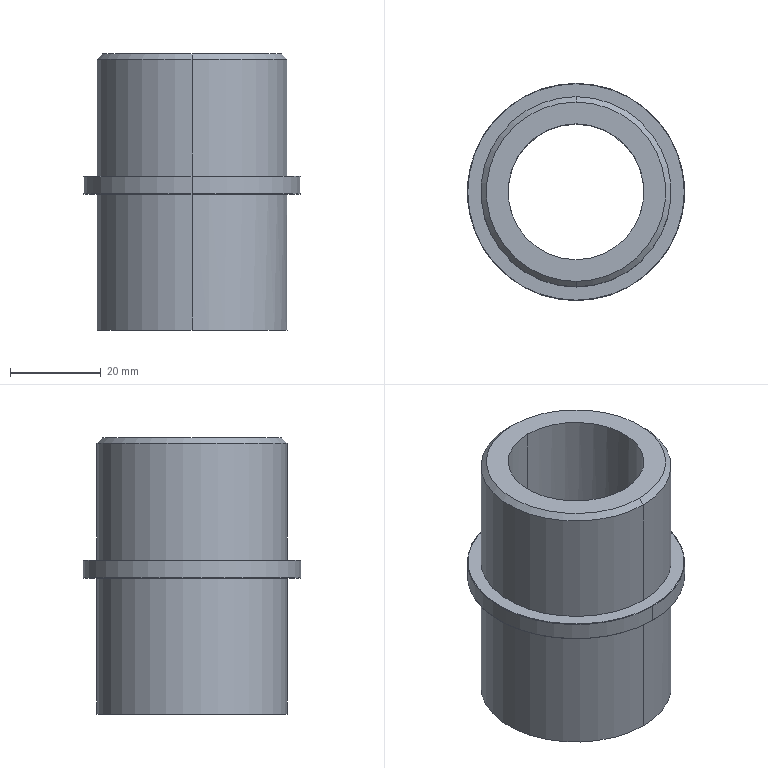Part | Creo | 1 solid | 18 faces | box 48 x 48 x 61 mm | volume 42995 mm3 | cylinder 8 | cone 6 | plane 4 | commonest cylinder face diameters 42 x4 30 x2 48 x2
STEP:
#1=CARTESIAN_POINT('',(166.,209.995,-326.));
#2=VERTEX_POINT('',#1);
#3=CARTESIAN_POINT('',(145.,188.995,-326.));
#4=VERTEX_POINT('',#3);
#5=CARTESIAN_POINT('',(145.,209.995,-326.));
#6=DIRECTION('',(0.,0.,-1.));
#7=DIRECTION('',(1.,0.,0.));
#8=AXIS2_PLACEMENT_3D('',#5,#6,#7);
#9=CIRCLE('',#8,21.);
#10=EDGE_CURVE('',#2,#4,#9,.T.);
#11=ORIENTED_EDGE('',*,*,#10,.F.);
#12=CARTESIAN_POINT('',(145.,230.995,-326.));
#13=VERTEX_POINT('',#12);
#14=CARTESIAN_POINT('',(145.,209.995,-326.));
#15=DIRECTION('',(0.,0.,-1.));
#16=DIRECTION('',(0.,1.,0.));
#17=AXIS2_PLACEMENT_3D('',#14,#15,#16);
#18=CIRCLE('',#17,21.);
#19=EDGE_CURVE('',#13,#2,#18,.T.);
#20=ORIENTED_EDGE('',*,*,#19,.F.);
#21=CARTESIAN_POINT('',(145.,209.995,-326.));
#22=DIRECTION('',(0.,0.,-1.));
#23=DIRECTION('',(0.,-1.,0.));
#24=AXIS2_PLACEMENT_3D('',#21,#22,#23);
#25=CIRCLE('',#24,21.);
#26=EDGE_CURVE('',#4,#13,#25,.T.);
#27=ORIENTED_EDGE('',*,*,#26,.F.);
#28=EDGE_LOOP('',(#11,#20,#27));
#29=FACE_OUTER_BOUND('',#28,.F.);
#30=CARTESIAN_POINT('',(160.,209.995,-326.));
#31=VERTEX_POINT('',#30);
#32=CARTESIAN_POINT('',(145.,224.995,-326.));
#33=VERTEX_POINT('',#32);
#34=CARTESIAN_POINT('',(145.,209.995,-326.));
#35=DIRECTION('',(0.,0.,1.));
#36=DIRECTION('',(1.,0.,0.));
#37=AXIS2_PLACEMENT_3D('',#34,#35,#36);
#38=CIRCLE('',#37,15.);
#39=EDGE_CURVE('',#31,#33,#38,.T.);
#40=ORIENTED_EDGE('',*,*,#39,.F.);
#41=CARTESIAN_POINT('',(145.,194.995,-326.));
#42=VERTEX_POINT('',#41);
#43=CARTESIAN_POINT('',(145.,209.995,-326.));
#44=DIRECTION('',(0.,0.,1.));
#45=DIRECTION('',(0.,-1.,0.));
#46=AXIS2_PLACEMENT_3D('',#43,#44,#45);
#47=CIRCLE('',#46,15.);
#48=EDGE_CURVE('',#42,#31,#47,.T.);
#49=ORIENTED_EDGE('',*,*,#48,.F.);
#50=CARTESIAN_POINT('',(130.,209.995,-326.));
#51=VERTEX_POINT('',#50);
#52=CARTESIAN_POINT('',(145.,209.995,-326.));
#53=DIRECTION('',(0.,0.,1.));
#54=DIRECTION('',(-1.,0.,0.));
#55=AXIS2_PLACEMENT_3D('',#52,#53,#54);
#56=CIRCLE('',#55,15.);
#57=EDGE_CURVE('',#51,#42,#56,.T.);
#58=ORIENTED_EDGE('',*,*,#57,.F.);
#59=CARTESIAN_POINT('',(145.,209.995,-326.));
#60=DIRECTION('',(0.,0.,1.));
#61=DIRECTION('',(0.,1.,0.));
#62=AXIS2_PLACEMENT_3D('',#59,#60,#61);
#63=CIRCLE('',#62,15.);
#64=EDGE_CURVE('',#33,#51,#63,.T.);
#65=ORIENTED_EDGE('',*,*,#64,.F.);
#66=EDGE_LOOP('',(#40,#49,#58,#65));
#67=FACE_BOUND('',#66,.F.);
#68=CARTESIAN_POINT('',(45.,-0.004699,-326.));
#69=DIRECTION('',(0.,0.,1.));
#70=DIRECTION('',(0.,1.,0.));
#71=AXIS2_PLACEMENT_3D('',#68,#69,#70);
#72=PLANE('',#71);
#73=ADVANCED_FACE('',(#29,#67),#72,.F.);
#74=CARTESIAN_POINT('',(145.,188.995,-296.));
#75=VERTEX_POINT('',#74);
#76=CARTESIAN_POINT('',(145.,230.995,-296.));
#77=VERTEX_POINT('',#76);
#78=CARTESIAN_POINT('',(145.,209.995,-296.));
#79=DIRECTION('',(0.,0.,1.));
#80=DIRECTION('',(0.,-1.,0.));
#81=AXIS2_PLACEMENT_3D('',#78,#79,#80);
#82=CIRCLE('',#81,21.);
#83=EDGE_CURVE('',#75,#77,#82,.T.);
#84=ORIENTED_EDGE('',*,*,#83,.T.);
#85=CARTESIAN_POINT('',(145.,230.995,-296.));
#86=DIRECTION('',(0.,0.,-1.));
#87=VECTOR('',#86,30.);
#88=LINE('',#85,#87);
#89=EDGE_CURVE('',#77,#13,#88,.T.);
#90=ORIENTED_EDGE('',*,*,#89,.T.);
#91=ORIENTED_EDGE('',*,*,#19,.T.);
#92=ORIENTED_EDGE('',*,*,#10,.T.);
#93=CARTESIAN_POINT('',(145.,188.995,-296.));
#94=DIRECTION('',(0.,0.,-1.));
#95=VECTOR('',#94,30.);
#96=LINE('',#93,#95);
#97=EDGE_CURVE('',#75,#4,#96,.T.);
#98=ORIENTED_EDGE('',*,*,#97,.F.);
#99=EDGE_LOOP('',(#84,#90,#91,#92,#98));
#100=FACE_OUTER_BOUND('',#99,.F.);
#101=CARTESIAN_POINT('',(145.,209.995,-262.35));
#102=DIRECTION('',(0.,0.,-1.));
#103=DIRECTION('',(0.,-1.,0.));
#104=AXIS2_PLACEMENT_3D('',#101,#102,#103);
#105=CYLINDRICAL_SURFACE('',#104,21.);
#106=ADVANCED_FACE('',(#100),#105,.T.);
#107=CARTESIAN_POINT('',(145.,186.095,-296.));
#108=VERTEX_POINT('',#107);
#109=CARTESIAN_POINT('',(145.,233.895,-296.));
#110=VERTEX_POINT('',#109);
#111=CARTESIAN_POINT('',(145.,209.995,-296.));
#112=DIRECTION('',(0.,0.,-1.));
#113=DIRECTION('',(0.,-1.,0.));
#114=AXIS2_PLACEMENT_3D('',#111,#112,#113);
#115=CIRCLE('',#114,23.9);
#116=EDGE_CURVE('',#108,#110,#115,.T.);
#117=ORIENTED_EDGE('',*,*,#116,.F.);
#118=CARTESIAN_POINT('',(145.,209.995,-296.));
#119=DIRECTION('',(0.,0.,-1.));
#120=DIRECTION('',(0.,1.,0.));
#121=AXIS2_PLACEMENT_3D('',#118,#119,#120);
#122=CIRCLE('',#121,23.9);
#123=EDGE_CURVE('',#110,#108,#122,.T.);
#124=ORIENTED_EDGE('',*,*,#123,.F.);
#125=EDGE_LOOP('',(#117,#124));
#126=FACE_OUTER_BOUND('',#125,.F.);
#127=ORIENTED_EDGE('',*,*,#83,.F.);
#128=CARTESIAN_POINT('',(145.,209.995,-296.));
#129=DIRECTION('',(0.,0.,1.));
#130=DIRECTION('',(0.,1.,0.));
#131=AXIS2_PLACEMENT_3D('',#128,#129,#130);
#132=CIRCLE('',#131,21.);
#133=EDGE_CURVE('',#77,#75,#132,.T.);
#134=ORIENTED_EDGE('',*,*,#133,.F.);
#135=EDGE_LOOP('',(#127,#134));
#136=FACE_BOUND('',#135,.F.);
#137=CARTESIAN_POINT('',(145.,209.995,-296.));
#138=DIRECTION('',(0.,0.,-1.));
#139=DIRECTION('',(0.,-1.,0.));
#140=AXIS2_PLACEMENT_3D('',#137,#138,#139);
#141=PLANE('',#140);
#142=ADVANCED_FACE('',(#126,#136),#141,.T.);
#143=ORIENTED_EDGE('',*,*,#133,.T.);
#144=ORIENTED_EDGE('',*,*,#97,.T.);
#145=ORIENTED_EDGE('',*,*,#26,.T.);
#146=ORIENTED_EDGE('',*,*,#89,.F.);
#147=EDGE_LOOP('',(#143,#144,#145,#146));
#148=FACE_OUTER_BOUND('',#147,.F.);
#149=CARTESIAN_POINT('',(145.,209.995,-262.35));
#150=DIRECTION('',(0.,0.,-1.));
#151=DIRECTION('',(0.,-1.,0.));
#152=AXIS2_PLACEMENT_3D('',#149,#150,#151);
#153=CYLINDRICAL_SURFACE('',#152,21.);
#154=ADVANCED_FACE('',(#148),#153,.T.);
#155=CARTESIAN_POINT('',(145.,185.995,-295.9));
#156=VERTEX_POINT('',#155);
#157=CARTESIAN_POINT('',(145.,233.995,-295.9));
#158=VERTEX_POINT('',#157);
#159=CARTESIAN_POINT('',(145.,209.995,-295.9));
#160=DIRECTION('',(0.,0.,-1.));
#161=DIRECTION('',(0.,-1.,0.));
#162=AXIS2_PLACEMENT_3D('',#159,#160,#161);
#163=CIRCLE('',#162,24.);
#164=EDGE_CURVE('',#156,#158,#163,.T.);
#165=ORIENTED_EDGE('',*,*,#164,.F.);
#166=CARTESIAN_POINT('',(145.,186.095,-296.));
#167=DIRECTION('',(0.,-0.7071,0.7071));
#168=VECTOR('',#167,0.1414);
#169=LINE('',#166,#168);
#170=EDGE_CURVE('',#108,#156,#169,.T.);
#171=ORIENTED_EDGE('',*,*,#170,.F.);
#172=ORIENTED_EDGE('',*,*,#116,.T.);
#173=CARTESIAN_POINT('',(145.,233.895,-296.));
#174=DIRECTION('',(0.,0.7071,0.7071));
#175=VECTOR('',#174,0.1414);
#176=LINE('',#173,#175);
#177=EDGE_CURVE('',#110,#158,#176,.T.);
#178=ORIENTED_EDGE('',*,*,#177,.T.);
#179=EDGE_LOOP('',(#165,#171,#172,#178));
#180=FACE_OUTER_BOUND('',#179,.F.);
#181=CARTESIAN_POINT('',(145.,209.995,-295.95));
#182=DIRECTION('',(0.,0.,1.));
#183=DIRECTION('',(0.,1.,0.));
#184=AXIS2_PLACEMENT_3D('',#181,#182,#183);
#185=CONICAL_SURFACE('',#184,23.95,45.);
#186=ADVANCED_FACE('',(#180),#185,.T.);
#187=CARTESIAN_POINT('',(145.,233.995,-292.1));
#188=VERTEX_POINT('',#187);
#189=CARTESIAN_POINT('',(145.,185.995,-292.1));
#190=VERTEX_POINT('',#189);
#191=CARTESIAN_POINT('',(145.,209.995,-292.1));
#192=DIRECTION('',(0.,0.,1.));
#193=DIRECTION('',(0.,1.,0.));
#194=AXIS2_PLACEMENT_3D('',#191,#192,#193);
#195=CIRCLE('',#194,24.);
#196=EDGE_CURVE('',#188,#190,#195,.T.);
#197=ORIENTED_EDGE('',*,*,#196,.T.);
#198=CARTESIAN_POINT('',(145.,185.995,-292.1));
#199=DIRECTION('',(0.,0.,-1.));
#200=VECTOR('',#199,3.8);
#201=LINE('',#198,#200);
#202=EDGE_CURVE('',#190,#156,#201,.T.);
#203=ORIENTED_EDGE('',*,*,#202,.T.);
#204=ORIENTED_EDGE('',*,*,#164,.T.);
#205=CARTESIAN_POINT('',(145.,233.995,-292.1));
#206=DIRECTION('',(0.,0.,-1.));
#207=VECTOR('',#206,3.8);
#208=LINE('',#205,#207);
#209=EDGE_CURVE('',#188,#158,#208,.T.);
#210=ORIENTED_EDGE('',*,*,#209,.F.);
#211=EDGE_LOOP('',(#197,#203,#204,#210));
#212=FACE_OUTER_BOUND('',#211,.F.);
#213=CARTESIAN_POINT('',(145.,209.995,-262.35));
#214=DIRECTION('',(0.,0.,-1.));
#215=DIRECTION('',(0.,-1.,0.));
#216=AXIS2_PLACEMENT_3D('',#213,#214,#215);
#217=CYLINDRICAL_SURFACE('',#216,24.);
#218=ADVANCED_FACE('',(#212),#217,.T.);
#219=ORIENTED_EDGE('',*,*,#196,.F.);
#220=CARTESIAN_POINT('',(145.,233.895,-292.));
#221=VERTEX_POINT('',#220);
#222=CARTESIAN_POINT('',(145.,233.895,-292.));
#223=DIRECTION('',(0.,0.7071,-0.7071));
#224=VECTOR('',#223,0.1414);
#225=LINE('',#222,#224);
#226=EDGE_CURVE('',#221,#188,#225,.T.);
#227=ORIENTED_EDGE('',*,*,#226,.F.);
#228=CARTESIAN_POINT('',(145.,186.095,-292.));
#229=VERTEX_POINT('',#228);
#230=CARTESIAN_POINT('',(145.,209.995,-292.));
#231=DIRECTION('',(0.,0.,1.));
#232=DIRECTION('',(0.,1.,0.));
#233=AXIS2_PLACEMENT_3D('',#230,#231,#232);
#234=CIRCLE('',#233,23.9);
#235=EDGE_CURVE('',#221,#229,#234,.T.);
#236=ORIENTED_EDGE('',*,*,#235,.T.);
#237=CARTESIAN_POINT('',(145.,186.095,-292.));
#238=DIRECTION('',(0.,-0.7071,-0.7071));
#239=VECTOR('',#238,0.1414);
#240=LINE('',#237,#239);
#241=EDGE_CURVE('',#229,#190,#240,.T.);
#242=ORIENTED_EDGE('',*,*,#241,.T.);
#243=EDGE_LOOP('',(#219,#227,#236,#242));
#244=FACE_OUTER_BOUND('',#243,.F.);
#245=CARTESIAN_POINT('',(145.,209.995,-292.05));
#246=DIRECTION('',(0.,0.,-1.));
#247=DIRECTION('',(0.,-1.,0.));
#248=AXIS2_PLACEMENT_3D('',#245,#246,#247);
#249=CONICAL_SURFACE('',#248,23.95,45.);
#250=ADVANCED_FACE('',(#244),#249,.T.);
#251=CARTESIAN_POINT('',(145.,209.995,-292.1));
#252=DIRECTION('',(0.,0.,1.));
#253=DIRECTION('',(0.,-1.,0.));
#254=AXIS2_PLACEMENT_3D('',#251,#252,#253);
#255=CIRCLE('',#254,24.);
#256=EDGE_CURVE('',#190,#188,#255,.T.);
#257=ORIENTED_EDGE('',*,*,#256,.F.);
#258=ORIENTED_EDGE('',*,*,#241,.F.);
#259=CARTESIAN_POINT('',(145.,209.995,-292.));
#260=DIRECTION('',(0.,0.,1.));
#261=DIRECTION('',(0.,-1.,0.));
#262=AXIS2_PLACEMENT_3D('',#259,#260,#261);
#263=CIRCLE('',#262,23.9);
#264=EDGE_CURVE('',#229,#221,#263,.T.);
#265=ORIENTED_EDGE('',*,*,#264,.T.);
#266=ORIENTED_EDGE('',*,*,#226,.T.);
#267=EDGE_LOOP('',(#257,#258,#265,#266));
#268=FACE_OUTER_BOUND('',#267,.F.);
#269=CARTESIAN_POINT('',(145.,209.995,-292.05));
#270=DIRECTION('',(0.,0.,-1.));
#271=DIRECTION('',(0.,-1.,0.));
#272=AXIS2_PLACEMENT_3D('',#269,#270,#271);
#273=CONICAL_SURFACE('',#272,23.95,45.);
#274=ADVANCED_FACE('',(#268),#273,.T.);
#275=ORIENTED_EDGE('',*,*,#256,.T.);
#276=ORIENTED_EDGE('',*,*,#209,.T.);
#277=CARTESIAN_POINT('',(145.,209.995,-295.9));
#278=DIRECTION('',(0.,0.,-1.));
#279=DIRECTION('',(0.,1.,0.));
#280=AXIS2_PLACEMENT_3D('',#277,#278,#279);
#281=CIRCLE('',#280,24.);
#282=EDGE_CURVE('',#158,#156,#281,.T.);
#283=ORIENTED_EDGE('',*,*,#282,.T.);
#284=ORIENTED_EDGE('',*,*,#202,.F.);
#285=EDGE_LOOP('',(#275,#276,#283,#284));
#286=FACE_OUTER_BOUND('',#285,.F.);
#287=CARTESIAN_POINT('',(145.,209.995,-262.35));
#288=DIRECTION('',(0.,0.,-1.));
#289=DIRECTION('',(0.,-1.,0.));
#290=AXIS2_PLACEMENT_3D('',#287,#288,#289);
#291=CYLINDRICAL_SURFACE('',#290,24.);
#292=ADVANCED_FACE('',(#286),#291,.T.);
#293=ORIENTED_EDGE('',*,*,#282,.F.);
#294=ORIENTED_EDGE('',*,*,#177,.F.);
#295=ORIENTED_EDGE('',*,*,#123,.T.);
#296=ORIENTED_EDGE('',*,*,#170,.T.);
#297=EDGE_LOOP('',(#293,#294,#295,#296));
#298=FACE_OUTER_BOUND('',#297,.F.);
#299=CARTESIAN_POINT('',(145.,209.995,-295.95));
#300=DIRECTION('',(0.,0.,1.));
#301=DIRECTION('',(0.,1.,0.));
#302=AXIS2_PLACEMENT_3D('',#299,#300,#301);
#303=CONICAL_SURFACE('',#302,23.95,45.);
#304=ADVANCED_FACE('',(#298),#303,.T.);
#305=ORIENTED_EDGE('',*,*,#264,.F.);
#306=ORIENTED_EDGE('',*,*,#235,.F.);
#307=EDGE_LOOP('',(#305,#306));
#308=FACE_OUTER_BOUND('',#307,.F.);
#309=CARTESIAN_POINT('',(145.,188.995,-292.));
#310=VERTEX_POINT('',#309);
#311=CARTESIAN_POINT('',(145.,230.995,-292.));
#312=VERTEX_POINT('',#311);
#313=CARTESIAN_POINT('',(145.,209.995,-292.));
#314=DIRECTION('',(0.,0.,-1.));
#315=DIRECTION('',(0.,-1.,0.));
#316=AXIS2_PLACEMENT_3D('',#313,#314,#315);
#317=CIRCLE('',#316,21.);
#318=EDGE_CURVE('',#310,#312,#317,.T.);
#319=ORIENTED_EDGE('',*,*,#318,.F.);
#320=CARTESIAN_POINT('',(145.,209.995,-292.));
#321=DIRECTION('',(0.,0.,-1.));
#322=DIRECTION('',(0.,1.,0.));
#323=AXIS2_PLACEMENT_3D('',#320,#321,#322);
#324=CIRCLE('',#323,21.);
#325=EDGE_CURVE('',#312,#310,#324,.T.);
#326=ORIENTED_EDGE('',*,*,#325,.F.);
#327=EDGE_LOOP('',(#319,#326));
#328=FACE_BOUND('',#327,.F.);
#329=CARTESIAN_POINT('',(145.,209.995,-292.));
#330=DIRECTION('',(0.,0.,-1.));
#331=DIRECTION('',(0.,-1.,0.));
#332=AXIS2_PLACEMENT_3D('',#329,#330,#331);
#333=PLANE('',#332);
#334=ADVANCED_FACE('',(#308,#328),#333,.F.);
#335=CARTESIAN_POINT('',(145.,230.995,-266.2));
#336=VERTEX_POINT('',#335);
#337=CARTESIAN_POINT('',(145.,188.995,-266.2));
#338=VERTEX_POINT('',#337);
#339=CARTESIAN_POINT('',(145.,209.995,-266.2));
#340=DIRECTION('',(0.,0.,1.));
#341=DIRECTION('',(0.,1.,0.));
#342=AXIS2_PLACEMENT_3D('',#339,#340,#341);
#343=CIRCLE('',#342,21.);
#344=EDGE_CURVE('',#336,#338,#343,.T.);
#345=ORIENTED_EDGE('',*,*,#344,.T.);
#346=CARTESIAN_POINT('',(145.,188.995,-266.2));
#347=DIRECTION('',(0.,0.,-1.));
#348=VECTOR('',#347,25.8);
#349=LINE('',#346,#348);
#350=EDGE_CURVE('',#338,#310,#349,.T.);
#351=ORIENTED_EDGE('',*,*,#350,.T.);
#352=ORIENTED_EDGE('',*,*,#318,.T.);
#353=CARTESIAN_POINT('',(145.,230.995,-266.2));
#354=DIRECTION('',(0.,0.,-1.));
#355=VECTOR('',#354,25.8);
#356=LINE('',#353,#355);
#357=EDGE_CURVE('',#336,#312,#356,.T.);
#358=ORIENTED_EDGE('',*,*,#357,.F.);
#359=EDGE_LOOP('',(#345,#351,#352,#358));
#360=FACE_OUTER_BOUND('',#359,.F.);
#361=CARTESIAN_POINT('',(145.,209.995,-262.35));
#362=DIRECTION('',(0.,0.,-1.));
#363=DIRECTION('',(0.,-1.,0.));
#364=AXIS2_PLACEMENT_3D('',#361,#362,#363);
#365=CYLINDRICAL_SURFACE('',#364,21.);
#366=ADVANCED_FACE('',(#360),#365,.T.);
#367=ORIENTED_EDGE('',*,*,#344,.F.);
#368=CARTESIAN_POINT('',(145.,229.795,-265.));
#369=VERTEX_POINT('',#368);
#370=CARTESIAN_POINT('',(145.,229.795,-265.));
#371=DIRECTION('',(0.,0.7071,-0.7071));
#372=VECTOR('',#371,1.697);
#373=LINE('',#370,#372);
#374=EDGE_CURVE('',#369,#336,#373,.T.);
#375=ORIENTED_EDGE('',*,*,#374,.F.);
#376=CARTESIAN_POINT('',(145.,190.195,-265.));
#377=VERTEX_POINT('',#376);
#378=CARTESIAN_POINT('',(145.,209.995,-265.));
#379=DIRECTION('',(0.,0.,1.));
#380=DIRECTION('',(0.,1.,0.));
#381=AXIS2_PLACEMENT_3D('',#378,#379,#380);
#382=CIRCLE('',#381,19.8);
#383=EDGE_CURVE('',#369,#377,#382,.T.);
#384=ORIENTED_EDGE('',*,*,#383,.T.);
#385=CARTESIAN_POINT('',(145.,190.195,-265.));
#386=DIRECTION('',(0.,-0.7071,-0.7071));
#387=VECTOR('',#386,1.697);
#388=LINE('',#385,#387);
#389=EDGE_CURVE('',#377,#338,#388,.T.);
#390=ORIENTED_EDGE('',*,*,#389,.T.);
#391=EDGE_LOOP('',(#367,#375,#384,#390));
#392=FACE_OUTER_BOUND('',#391,.F.);
#393=CARTESIAN_POINT('',(145.,209.995,-265.6));
#394=DIRECTION('',(0.,0.,-1.));
#395=DIRECTION('',(0.,-1.,0.));
#396=AXIS2_PLACEMENT_3D('',#393,#394,#395);
#397=CONICAL_SURFACE('',#396,20.4,45.);
#398=ADVANCED_FACE('',(#392),#397,.T.);
#399=CARTESIAN_POINT('',(145.,209.995,-266.2));
#400=DIRECTION('',(0.,0.,1.));
#401=DIRECTION('',(0.,-1.,0.));
#402=AXIS2_PLACEMENT_3D('',#399,#400,#401);
#403=CIRCLE('',#402,21.);
#404=EDGE_CURVE('',#338,#336,#403,.T.);
#405=ORIENTED_EDGE('',*,*,#404,.F.);
#406=ORIENTED_EDGE('',*,*,#389,.F.);
#407=CARTESIAN_POINT('',(145.,209.995,-265.));
#408=DIRECTION('',(0.,0.,1.));
#409=DIRECTION('',(0.,-1.,0.));
#410=AXIS2_PLACEMENT_3D('',#407,#408,#409);
#411=CIRCLE('',#410,19.8);
#412=EDGE_CURVE('',#377,#369,#411,.T.);
#413=ORIENTED_EDGE('',*,*,#412,.T.);
#414=ORIENTED_EDGE('',*,*,#374,.T.);
#415=EDGE_LOOP('',(#405,#406,#413,#414));
#416=FACE_OUTER_BOUND('',#415,.F.);
#417=CARTESIAN_POINT('',(145.,209.995,-265.6));
#418=DIRECTION('',(0.,0.,-1.));
#419=DIRECTION('',(0.,-1.,0.));
#420=AXIS2_PLACEMENT_3D('',#417,#418,#419);
#421=CONICAL_SURFACE('',#420,20.4,45.);
#422=ADVANCED_FACE('',(#416),#421,.T.);
#423=ORIENTED_EDGE('',*,*,#404,.T.);
#424=ORIENTED_EDGE('',*,*,#357,.T.);
#425=ORIENTED_EDGE('',*,*,#325,.T.);
#426=ORIENTED_EDGE('',*,*,#350,.F.);
#427=EDGE_LOOP('',(#423,#424,#425,#426));
#428=FACE_OUTER_BOUND('',#427,.F.);
#429=CARTESIAN_POINT('',(145.,209.995,-262.35));
#430=DIRECTION('',(0.,0.,-1.));
#431=DIRECTION('',(0.,-1.,0.));
#432=AXIS2_PLACEMENT_3D('',#429,#430,#431);
#433=CYLINDRICAL_SURFACE('',#432,21.);
#434=ADVANCED_FACE('',(#428),#433,.T.);
#435=ORIENTED_EDGE('',*,*,#412,.F.);
#436=ORIENTED_EDGE('',*,*,#383,.F.);
#437=EDGE_LOOP('',(#435,#436));
#438=FACE_OUTER_BOUND('',#437,.F.);
#439=CARTESIAN_POINT('',(145.,194.995,-265.));
#440=VERTEX_POINT('',#439);
#441=CARTESIAN_POINT('',(145.,224.995,-265.));
#442=VERTEX_POINT('',#441);
#443=CARTESIAN_POINT('',(145.,209.995,-265.));
#444=DIRECTION('',(0.,0.,-1.));
#445=DIRECTION('',(0.,-1.,0.));
#446=AXIS2_PLACEMENT_3D('',#443,#444,#445);
#447=CIRCLE('',#446,15.);
#448=EDGE_CURVE('',#440,#442,#447,.T.);
#449=ORIENTED_EDGE('',*,*,#448,.F.);
#450=CARTESIAN_POINT('',(145.,209.995,-265.));
#451=DIRECTION('',(0.,0.,-1.));
#452=DIRECTION('',(0.,1.,0.));
#453=AXIS2_PLACEMENT_3D('',#450,#451,#452);
#454=CIRCLE('',#453,15.);
#455=EDGE_CURVE('',#442,#440,#454,.T.);
#456=ORIENTED_EDGE('',*,*,#455,.F.);
#457=EDGE_LOOP('',(#449,#456));
#458=FACE_BOUND('',#457,.F.);
#459=CARTESIAN_POINT('',(145.,209.995,-265.));
#460=DIRECTION('',(0.,0.,-1.));
#461=DIRECTION('',(0.,-1.,0.));
#462=AXIS2_PLACEMENT_3D('',#459,#460,#461);
#463=PLANE('',#462);
#464=ADVANCED_FACE('',(#438,#458),#463,.F.);
#465=ORIENTED_EDGE('',*,*,#57,.T.);
#466=CARTESIAN_POINT('',(145.,194.995,-265.));
#467=DIRECTION('',(0.,0.,-1.));
#468=VECTOR('',#467,61.);
#469=LINE('',#466,#468);
#470=EDGE_CURVE('',#440,#42,#469,.T.);
#471=ORIENTED_EDGE('',*,*,#470,.F.);
#472=ORIENTED_EDGE('',*,*,#448,.T.);
#473=CARTESIAN_POINT('',(145.,224.995,-265.));
#474=DIRECTION('',(0.,0.,-1.));
#475=VECTOR('',#474,61.);
#476=LINE('',#473,#475);
#477=EDGE_CURVE('',#442,#33,#476,.T.);
#478=ORIENTED_EDGE('',*,*,#477,.T.);
#479=ORIENTED_EDGE('',*,*,#64,.T.);
#480=EDGE_LOOP('',(#465,#471,#472,#478,#479));
#481=FACE_OUTER_BOUND('',#480,.F.);
#482=CARTESIAN_POINT('',(145.,209.995,-262.35));
#483=DIRECTION('',(0.,0.,-1.));
#484=DIRECTION('',(0.,-1.,0.));
#485=AXIS2_PLACEMENT_3D('',#482,#483,#484);
#486=CYLINDRICAL_SURFACE('',#485,15.);
#487=ADVANCED_FACE('',(#481),#486,.F.);
#488=ORIENTED_EDGE('',*,*,#48,.T.);
#489=ORIENTED_EDGE('',*,*,#39,.T.);
#490=ORIENTED_EDGE('',*,*,#477,.F.);
#491=ORIENTED_EDGE('',*,*,#455,.T.);
#492=ORIENTED_EDGE('',*,*,#470,.T.);
#493=EDGE_LOOP('',(#488,#489,#490,#491,#492));
#494=FACE_OUTER_BOUND('',#493,.F.);
#495=CARTESIAN_POINT('',(145.,209.995,-262.35));
#496=DIRECTION('',(0.,0.,-1.));
#497=DIRECTION('',(0.,-1.,0.));
#498=AXIS2_PLACEMENT_3D('',#495,#496,#497);
#499=CYLINDRICAL_SURFACE('',#498,15.);
#500=ADVANCED_FACE('',(#494),#499,.F.);
#501=CLOSED_SHELL('',(#73,#106,#142,#154,#186,#218,#250,#274,#292,#304,#334,#366,#398,#422,#434,#464,#487,#500));
#502=MANIFOLD_SOLID_BREP('',#501);
#503=(LENGTH_UNIT()NAMED_UNIT(*)SI_UNIT(.MILLI.,.METRE.));
#504=UNCERTAINTY_MEASURE_WITH_UNIT(LENGTH_MEASURE(0.009126),#503,'','');
#505=(NAMED_UNIT(*)PLANE_ANGLE_UNIT()SI_UNIT($,.RADIAN.));
#506=PLANE_ANGLE_MEASURE_WITH_UNIT(PLANE_ANGLE_MEASURE(0.01745),#505);
#507=(CONVERSION_BASED_UNIT('DEGREE',#506)NAMED_UNIT(*)PLANE_ANGLE_UNIT());
#508=(NAMED_UNIT(*)SI_UNIT($,.STERADIAN.)SOLID_ANGLE_UNIT());
#509=(GEOMETRIC_REPRESENTATION_CONTEXT(3)GLOBAL_UNCERTAINTY_ASSIGNED_CONTEXT((#504))GLOBAL_UNIT_ASSIGNED_CONTEXT((#503,#507,#508))REPRESENTATION_CONTEXT('',''));
#510=ADVANCED_BREP_SHAPE_REPRESENTATION('',(#502),#509);